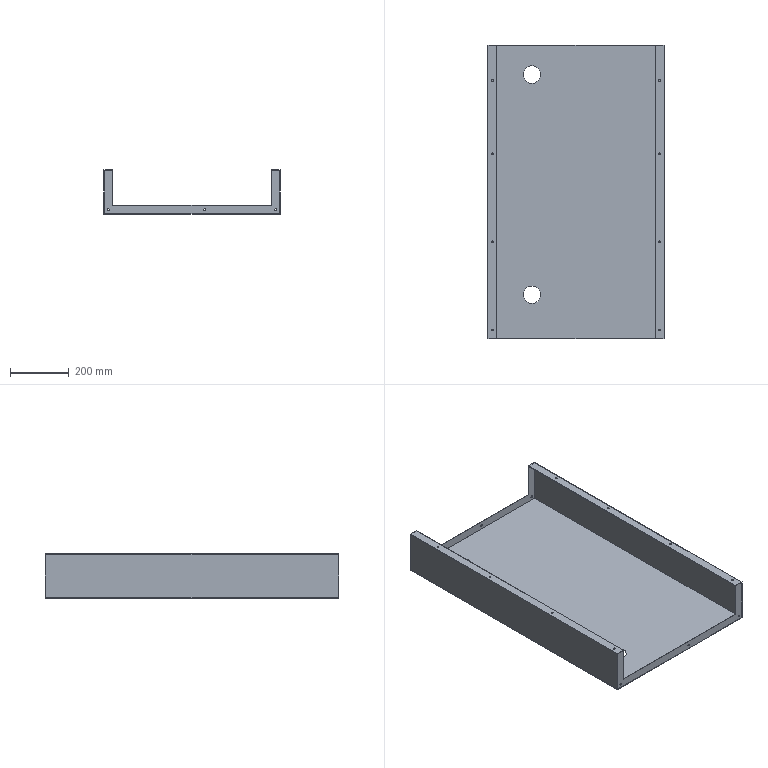Part | SolidWorks | features ICE 7, Extrusion 1, Shell 1 | 1 solid | 50 faces | box 600 x 1000 x 150 mm | volume 1985083 mm3 | cylinder 32 | plane 18 | commonest cylinder face diameters 6 x28 60 x4